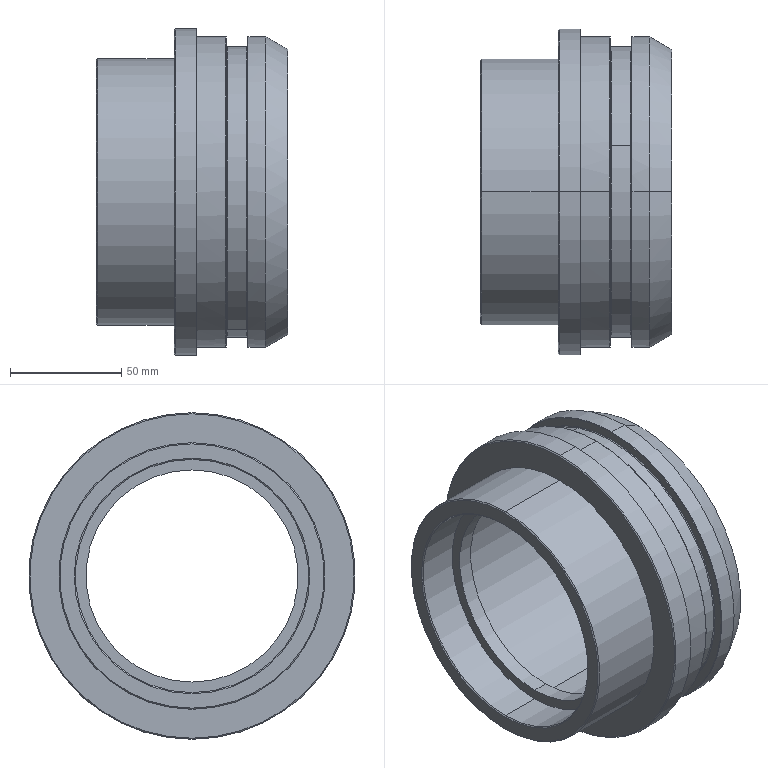Part | SolidWorks | features ICE 5, Chamfer 3, Cavity 1, Extrusion 1 | 1 solid | 42 faces | box 86 x 147 x 147 mm | volume 431094 mm3 | cylinder 16 | cone 10 | torus 8 | plane 8 | commonest cylinder face diameters 105 x4 140 x4 95.5 x2 120 x2 131 x2 147 x2
STEP:
#1=CARTESIAN_POINT('',(0.,0.,59.5));
#2=VERTEX_POINT('',#1);
#3=CARTESIAN_POINT('',(0.,0.,-59.5));
#4=VERTEX_POINT('',#3);
#5=CARTESIAN_POINT('',(0.,0.,0.));
#6=DIRECTION('',(-1.,0.,0.));
#7=DIRECTION('',(0.,0.,-1.));
#8=AXIS2_PLACEMENT_3D('',#5,#6,#7);
#9=CIRCLE('',#8,59.5);
#10=EDGE_CURVE('',#2,#4,#9,.T.);
#11=ORIENTED_EDGE('',*,*,#10,.F.);
#12=CARTESIAN_POINT('',(0.5,0.,60.));
#13=VERTEX_POINT('',#12);
#14=CARTESIAN_POINT('',(0.,0.,59.5));
#15=DIRECTION('',(0.7071,0.,0.7071));
#16=VECTOR('',#15,1000.);
#17=LINE('',#14,#16);
#18=EDGE_CURVE('',#2,#13,#17,.T.);
#19=ORIENTED_EDGE('',*,*,#18,.T.);
#20=CARTESIAN_POINT('',(0.5,0.,-60.));
#21=VERTEX_POINT('',#20);
#22=CARTESIAN_POINT('',(0.5,0.,0.));
#23=DIRECTION('',(1.,0.,0.));
#24=DIRECTION('',(0.,0.,-1.));
#25=AXIS2_PLACEMENT_3D('',#22,#23,#24);
#26=CIRCLE('',#25,60.);
#27=EDGE_CURVE('',#21,#13,#26,.T.);
#28=ORIENTED_EDGE('',*,*,#27,.F.);
#29=CARTESIAN_POINT('',(0.,0.,-59.5));
#30=DIRECTION('',(0.7071,0.,-0.7071));
#31=VECTOR('',#30,1000.);
#32=LINE('',#29,#31);
#33=EDGE_CURVE('',#4,#21,#32,.T.);
#34=ORIENTED_EDGE('',*,*,#33,.F.);
#35=EDGE_LOOP('',(#11,#19,#28,#34));
#36=FACE_OUTER_BOUND('',#35,.T.);
#37=CARTESIAN_POINT('',(0.,0.,0.));
#38=DIRECTION('',(1.,0.,0.));
#39=DIRECTION('',(0.,0.,-1.));
#40=AXIS2_PLACEMENT_3D('',#37,#38,#39);
#41=CONICAL_SURFACE('',#40,59.5,0.7854);
#42=ADVANCED_FACE('',(#36),#41,.T.);
#43=CARTESIAN_POINT('',(35.,0.,73.));
#44=VERTEX_POINT('',#43);
#45=CARTESIAN_POINT('',(35.,0.,-73.));
#46=VERTEX_POINT('',#45);
#47=CARTESIAN_POINT('',(35.,0.,0.));
#48=DIRECTION('',(-1.,0.,0.));
#49=DIRECTION('',(0.,0.,1.));
#50=AXIS2_PLACEMENT_3D('',#47,#48,#49);
#51=CIRCLE('',#50,73.);
#52=EDGE_CURVE('',#44,#46,#51,.T.);
#53=ORIENTED_EDGE('',*,*,#52,.F.);
#54=CARTESIAN_POINT('',(35.5,0.,73.5));
#55=VERTEX_POINT('',#54);
#56=CARTESIAN_POINT('',(35.,0.,73.));
#57=DIRECTION('',(0.7071,0.,0.7071));
#58=VECTOR('',#57,1000.);
#59=LINE('',#56,#58);
#60=EDGE_CURVE('',#44,#55,#59,.T.);
#61=ORIENTED_EDGE('',*,*,#60,.T.);
#62=CARTESIAN_POINT('',(35.5,0.,-73.5));
#63=VERTEX_POINT('',#62);
#64=CARTESIAN_POINT('',(35.5,0.,0.));
#65=DIRECTION('',(1.,0.,0.));
#66=DIRECTION('',(0.,0.,1.));
#67=AXIS2_PLACEMENT_3D('',#64,#65,#66);
#68=CIRCLE('',#67,73.5);
#69=EDGE_CURVE('',#63,#55,#68,.T.);
#70=ORIENTED_EDGE('',*,*,#69,.F.);
#71=CARTESIAN_POINT('',(35.,0.,-73.));
#72=DIRECTION('',(0.7071,0.,-0.7071));
#73=VECTOR('',#72,1000.);
#74=LINE('',#71,#73);
#75=EDGE_CURVE('',#46,#63,#74,.T.);
#76=ORIENTED_EDGE('',*,*,#75,.F.);
#77=EDGE_LOOP('',(#53,#61,#70,#76));
#78=FACE_OUTER_BOUND('',#77,.T.);
#79=CARTESIAN_POINT('',(35.,0.,0.));
#80=DIRECTION('',(1.,0.,0.));
#81=DIRECTION('',(0.,0.,-1.));
#82=AXIS2_PLACEMENT_3D('',#79,#80,#81);
#83=CONICAL_SURFACE('',#82,73.,0.7854);
#84=ADVANCED_FACE('',(#78),#83,.T.);
#85=CARTESIAN_POINT('',(0.5,0.,-52.5));
#86=VERTEX_POINT('',#85);
#87=CARTESIAN_POINT('',(0.5,0.,52.5));
#88=VERTEX_POINT('',#87);
#89=CARTESIAN_POINT('',(0.5,0.,0.));
#90=DIRECTION('',(-1.,0.,0.));
#91=DIRECTION('',(0.,0.,-1.));
#92=AXIS2_PLACEMENT_3D('',#89,#90,#91);
#93=CIRCLE('',#92,52.5);
#94=EDGE_CURVE('',#86,#88,#93,.T.);
#95=ORIENTED_EDGE('',*,*,#94,.F.);
#96=CARTESIAN_POINT('',(0.,0.,-53.));
#97=VERTEX_POINT('',#96);
#98=CARTESIAN_POINT('',(0.5,0.,-52.5));
#99=DIRECTION('',(-0.7071,0.,-0.7071));
#100=VECTOR('',#99,1000.);
#101=LINE('',#98,#100);
#102=EDGE_CURVE('',#86,#97,#101,.T.);
#103=ORIENTED_EDGE('',*,*,#102,.T.);
#104=CARTESIAN_POINT('',(0.,0.,53.));
#105=VERTEX_POINT('',#104);
#106=CARTESIAN_POINT('',(0.,0.,0.));
#107=DIRECTION('',(1.,0.,0.));
#108=DIRECTION('',(0.,0.,-1.));
#109=AXIS2_PLACEMENT_3D('',#106,#107,#108);
#110=CIRCLE('',#109,53.);
#111=EDGE_CURVE('',#105,#97,#110,.T.);
#112=ORIENTED_EDGE('',*,*,#111,.F.);
#113=CARTESIAN_POINT('',(0.5,0.,52.5));
#114=DIRECTION('',(-0.7071,0.,0.7071));
#115=VECTOR('',#114,1000.);
#116=LINE('',#113,#115);
#117=EDGE_CURVE('',#88,#105,#116,.T.);
#118=ORIENTED_EDGE('',*,*,#117,.F.);
#119=EDGE_LOOP('',(#95,#103,#112,#118));
#120=FACE_OUTER_BOUND('',#119,.T.);
#121=CARTESIAN_POINT('',(0.5,0.,0.));
#122=DIRECTION('',(-1.,0.,0.));
#123=DIRECTION('',(0.,0.,1.));
#124=AXIS2_PLACEMENT_3D('',#121,#122,#123);
#125=CONICAL_SURFACE('',#124,52.5,0.7854);
#126=ADVANCED_FACE('',(#120),#125,.F.);
#127=CARTESIAN_POINT('',(35.,0.,60.));
#128=VERTEX_POINT('',#127);
#129=CARTESIAN_POINT('',(35.,0.,-60.));
#130=VERTEX_POINT('',#129);
#131=CARTESIAN_POINT('',(35.,0.,0.));
#132=DIRECTION('',(-1.,0.,0.));
#133=DIRECTION('',(0.,0.,1.));
#134=AXIS2_PLACEMENT_3D('',#131,#132,#133);
#135=CIRCLE('',#134,60.);
#136=EDGE_CURVE('',#128,#130,#135,.T.);
#137=ORIENTED_EDGE('',*,*,#136,.T.);
#138=CARTESIAN_POINT('',(35.,0.,-60.));
#139=DIRECTION('',(-1.,0.,0.));
#140=VECTOR('',#139,1000.);
#141=LINE('',#138,#140);
#142=EDGE_CURVE('',#130,#21,#141,.T.);
#143=ORIENTED_EDGE('',*,*,#142,.T.);
#144=ORIENTED_EDGE('',*,*,#27,.T.);
#145=CARTESIAN_POINT('',(35.,0.,60.));
#146=DIRECTION('',(-1.,0.,0.));
#147=VECTOR('',#146,1000.);
#148=LINE('',#145,#147);
#149=EDGE_CURVE('',#128,#13,#148,.T.);
#150=ORIENTED_EDGE('',*,*,#149,.F.);
#151=EDGE_LOOP('',(#137,#143,#144,#150));
#152=FACE_OUTER_BOUND('',#151,.T.);
#153=CARTESIAN_POINT('',(35.,0.,0.));
#154=DIRECTION('',(-1.,0.,0.));
#155=DIRECTION('',(0.,0.,1.));
#156=AXIS2_PLACEMENT_3D('',#153,#154,#155);
#157=CYLINDRICAL_SURFACE('',#156,60.);
#158=ADVANCED_FACE('',(#152),#157,.T.);
#159=CARTESIAN_POINT('',(58.4,-22.387,-66.113));
#160=VERTEX_POINT('',#159);
#161=CARTESIAN_POINT('',(58.4,22.387,66.113));
#162=VERTEX_POINT('',#161);
#163=CARTESIAN_POINT('',(58.4,0.,0.));
#164=DIRECTION('',(-1.,0.,0.));
#165=DIRECTION('',(0.,-0.3207,-0.9472));
#166=AXIS2_PLACEMENT_3D('',#163,#164,#165);
#167=CIRCLE('',#166,69.8);
#168=EDGE_CURVE('',#160,#162,#167,.T.);
#169=ORIENTED_EDGE('',*,*,#168,.T.);
#170=CARTESIAN_POINT('',(58.2,22.451,66.302));
#171=VERTEX_POINT('',#170);
#172=CARTESIAN_POINT('',(58.2,22.387,66.113));
#173=DIRECTION('',(0.,-0.9472,0.3207));
#174=DIRECTION('',(0.,-0.3207,-0.9472));
#175=AXIS2_PLACEMENT_3D('',#172,#173,#174);
#176=CIRCLE('',#175,0.2);
#177=EDGE_CURVE('',#162,#171,#176,.T.);
#178=ORIENTED_EDGE('',*,*,#177,.T.);
#179=CARTESIAN_POINT('',(58.2,0.,70.));
#180=VERTEX_POINT('',#179);
#181=CARTESIAN_POINT('',(58.2,0.,0.));
#182=DIRECTION('',(-1.,0.,0.));
#183=DIRECTION('',(0.,-0.3207,-0.9472));
#184=AXIS2_PLACEMENT_3D('',#181,#182,#183);
#185=CIRCLE('',#184,70.);
#186=EDGE_CURVE('',#180,#171,#185,.T.);
#187=ORIENTED_EDGE('',*,*,#186,.F.);
#188=CARTESIAN_POINT('',(58.2,-22.451,-66.302));
#189=VERTEX_POINT('',#188);
#190=CARTESIAN_POINT('',(58.2,0.,0.));
#191=DIRECTION('',(-1.,0.,0.));
#192=DIRECTION('',(0.,-0.3207,-0.9472));
#193=AXIS2_PLACEMENT_3D('',#190,#191,#192);
#194=CIRCLE('',#193,70.);
#195=EDGE_CURVE('',#189,#180,#194,.T.);
#196=ORIENTED_EDGE('',*,*,#195,.F.);
#197=CARTESIAN_POINT('',(58.2,-22.387,-66.113));
#198=DIRECTION('',(0.,0.9472,-0.3207));
#199=DIRECTION('',(0.,0.3207,0.9472));
#200=AXIS2_PLACEMENT_3D('',#197,#198,#199);
#201=CIRCLE('',#200,0.2);
#202=EDGE_CURVE('',#160,#189,#201,.T.);
#203=ORIENTED_EDGE('',*,*,#202,.F.);
#204=EDGE_LOOP('',(#169,#178,#187,#196,#203));
#205=FACE_OUTER_BOUND('',#204,.T.);
#206=CARTESIAN_POINT('',(58.2,0.,0.));
#207=DIRECTION('',(-1.,0.,0.));
#208=DIRECTION('',(0.,-0.3207,-0.9472));
#209=AXIS2_PLACEMENT_3D('',#206,#207,#208);
#210=TOROIDAL_SURFACE('',#209,69.8,0.2);
#211=ADVANCED_FACE('',(#205),#210,.T.);
#212=CARTESIAN_POINT('',(68.2,0.,70.));
#213=VERTEX_POINT('',#212);
#214=CARTESIAN_POINT('',(68.2,22.451,66.302));
#215=VERTEX_POINT('',#214);
#216=CARTESIAN_POINT('',(68.2,0.,0.));
#217=DIRECTION('',(-1.,0.,0.));
#218=DIRECTION('',(0.,-0.3207,-0.9472));
#219=AXIS2_PLACEMENT_3D('',#216,#217,#218);
#220=CIRCLE('',#219,70.);
#221=EDGE_CURVE('',#213,#215,#220,.T.);
#222=ORIENTED_EDGE('',*,*,#221,.T.);
#223=CARTESIAN_POINT('',(68.,22.387,66.113));
#224=VERTEX_POINT('',#223);
#225=CARTESIAN_POINT('',(68.2,22.387,66.113));
#226=DIRECTION('',(0.,-0.9472,0.3207));
#227=DIRECTION('',(0.,-0.3207,-0.9472));
#228=AXIS2_PLACEMENT_3D('',#225,#226,#227);
#229=CIRCLE('',#228,0.2);
#230=EDGE_CURVE('',#215,#224,#229,.T.);
#231=ORIENTED_EDGE('',*,*,#230,.T.);
#232=CARTESIAN_POINT('',(68.,-22.387,-66.113));
#233=VERTEX_POINT('',#232);
#234=CARTESIAN_POINT('',(68.,0.,0.));
#235=DIRECTION('',(-1.,0.,0.));
#236=DIRECTION('',(0.,-0.3207,-0.9472));
#237=AXIS2_PLACEMENT_3D('',#234,#235,#236);
#238=CIRCLE('',#237,69.8);
#239=EDGE_CURVE('',#233,#224,#238,.T.);
#240=ORIENTED_EDGE('',*,*,#239,.F.);
#241=CARTESIAN_POINT('',(68.2,-22.451,-66.302));
#242=VERTEX_POINT('',#241);
#243=CARTESIAN_POINT('',(68.2,-22.387,-66.113));
#244=DIRECTION('',(0.,0.9472,-0.3207));
#245=DIRECTION('',(0.,0.3207,0.9472));
#246=AXIS2_PLACEMENT_3D('',#243,#244,#245);
#247=CIRCLE('',#246,0.2);
#248=EDGE_CURVE('',#242,#233,#247,.T.);
#249=ORIENTED_EDGE('',*,*,#248,.F.);
#250=CARTESIAN_POINT('',(68.2,0.,0.));
#251=DIRECTION('',(-1.,0.,0.));
#252=DIRECTION('',(0.,-0.3207,-0.9472));
#253=AXIS2_PLACEMENT_3D('',#250,#251,#252);
#254=CIRCLE('',#253,70.);
#255=EDGE_CURVE('',#242,#213,#254,.T.);
#256=ORIENTED_EDGE('',*,*,#255,.T.);
#257=EDGE_LOOP('',(#222,#231,#240,#249,#256));
#258=FACE_OUTER_BOUND('',#257,.T.);
#259=CARTESIAN_POINT('',(68.2,0.,0.));
#260=DIRECTION('',(-1.,0.,0.));
#261=DIRECTION('',(0.,-0.3207,-0.9472));
#262=AXIS2_PLACEMENT_3D('',#259,#260,#261);
#263=TOROIDAL_SURFACE('',#262,69.8,0.2);
#264=ADVANCED_FACE('',(#258),#263,.T.);
#265=CARTESIAN_POINT('',(67.6,21.007,62.04));
#266=VERTEX_POINT('',#265);
#267=CARTESIAN_POINT('',(67.6,-21.007,-62.04));
#268=VERTEX_POINT('',#267);
#269=CARTESIAN_POINT('',(67.6,0.,0.));
#270=DIRECTION('',(-1.,0.,0.));
#271=DIRECTION('',(0.,-0.3207,-0.9472));
#272=AXIS2_PLACEMENT_3D('',#269,#270,#271);
#273=CIRCLE('',#272,65.5);
#274=EDGE_CURVE('',#266,#268,#273,.T.);
#275=ORIENTED_EDGE('',*,*,#274,.F.);
#276=CARTESIAN_POINT('',(68.,21.136,62.419));
#277=VERTEX_POINT('',#276);
#278=CARTESIAN_POINT('',(67.6,21.136,62.419));
#279=DIRECTION('',(0.,-0.9472,0.3207));
#280=DIRECTION('',(0.,-0.3207,-0.9472));
#281=AXIS2_PLACEMENT_3D('',#278,#279,#280);
#282=CIRCLE('',#281,0.4);
#283=EDGE_CURVE('',#266,#277,#282,.T.);
#284=ORIENTED_EDGE('',*,*,#283,.T.);
#285=CARTESIAN_POINT('',(68.,-21.136,-62.419));
#286=VERTEX_POINT('',#285);
#287=CARTESIAN_POINT('',(68.,0.,0.));
#288=DIRECTION('',(-1.,0.,0.));
#289=DIRECTION('',(0.,-0.3207,-0.9472));
#290=AXIS2_PLACEMENT_3D('',#287,#288,#289);
#291=CIRCLE('',#290,65.9);
#292=EDGE_CURVE('',#277,#286,#291,.T.);
#293=ORIENTED_EDGE('',*,*,#292,.T.);
#294=CARTESIAN_POINT('',(67.6,-21.136,-62.419));
#295=DIRECTION('',(0.,0.9472,-0.3207));
#296=DIRECTION('',(0.,0.3207,0.9472));
#297=AXIS2_PLACEMENT_3D('',#294,#295,#296);
#298=CIRCLE('',#297,0.4);
#299=EDGE_CURVE('',#268,#286,#298,.T.);
#300=ORIENTED_EDGE('',*,*,#299,.F.);
#301=EDGE_LOOP('',(#275,#284,#293,#300));
#302=FACE_OUTER_BOUND('',#301,.T.);
#303=CARTESIAN_POINT('',(67.6,0.,0.));
#304=DIRECTION('',(-1.,0.,0.));
#305=DIRECTION('',(0.,-0.3207,-0.9472));
#306=AXIS2_PLACEMENT_3D('',#303,#304,#305);
#307=TOROIDAL_SURFACE('',#306,65.9,0.4);
#308=ADVANCED_FACE('',(#302),#307,.F.);
#309=CARTESIAN_POINT('',(58.4,21.136,62.419));
#310=VERTEX_POINT('',#309);
#311=CARTESIAN_POINT('',(58.4,-21.136,-62.419));
#312=VERTEX_POINT('',#311);
#313=CARTESIAN_POINT('',(58.4,0.,0.));
#314=DIRECTION('',(-1.,0.,0.));
#315=DIRECTION('',(0.,-0.3207,-0.9472));
#316=AXIS2_PLACEMENT_3D('',#313,#314,#315);
#317=CIRCLE('',#316,65.9);
#318=EDGE_CURVE('',#310,#312,#317,.T.);
#319=ORIENTED_EDGE('',*,*,#318,.F.);
#320=CARTESIAN_POINT('',(58.8,21.007,62.04));
#321=VERTEX_POINT('',#320);
#322=CARTESIAN_POINT('',(58.8,21.136,62.419));
#323=DIRECTION('',(0.,-0.9472,0.3207));
#324=DIRECTION('',(0.,-0.3207,-0.9472));
#325=AXIS2_PLACEMENT_3D('',#322,#323,#324);
#326=CIRCLE('',#325,0.4);
#327=EDGE_CURVE('',#310,#321,#326,.T.);
#328=ORIENTED_EDGE('',*,*,#327,.T.);
#329=CARTESIAN_POINT('',(58.8,-21.007,-62.04));
#330=VERTEX_POINT('',#329);
#331=CARTESIAN_POINT('',(58.8,0.,0.));
#332=DIRECTION('',(-1.,0.,0.));
#333=DIRECTION('',(0.,-0.3207,-0.9472));
#334=AXIS2_PLACEMENT_3D('',#331,#332,#333);
#335=CIRCLE('',#334,65.5);
#336=EDGE_CURVE('',#321,#330,#335,.T.);
#337=ORIENTED_EDGE('',*,*,#336,.T.);
#338=CARTESIAN_POINT('',(58.8,-21.136,-62.419));
#339=DIRECTION('',(0.,0.9472,-0.3207));
#340=DIRECTION('',(0.,0.3207,0.9472));
#341=AXIS2_PLACEMENT_3D('',#338,#339,#340);
#342=CIRCLE('',#341,0.4);
#343=EDGE_CURVE('',#312,#330,#342,.T.);
#344=ORIENTED_EDGE('',*,*,#343,.F.);
#345=EDGE_LOOP('',(#319,#328,#337,#344));
#346=FACE_OUTER_BOUND('',#345,.T.);
#347=CARTESIAN_POINT('',(58.8,0.,0.));
#348=DIRECTION('',(-1.,0.,0.));
#349=DIRECTION('',(0.,-0.3207,-0.9472));
#350=AXIS2_PLACEMENT_3D('',#347,#348,#349);
#351=TOROIDAL_SURFACE('',#350,65.9,0.4);
#352=ADVANCED_FACE('',(#346),#351,.F.);
#353=CARTESIAN_POINT('',(67.6,0.,0.));
#354=DIRECTION('',(-1.,0.,0.));
#355=DIRECTION('',(0.,-0.3207,-0.9472));
#356=AXIS2_PLACEMENT_3D('',#353,#354,#355);
#357=CIRCLE('',#356,65.5);
#358=EDGE_CURVE('',#268,#266,#357,.T.);
#359=ORIENTED_EDGE('',*,*,#358,.T.);
#360=CARTESIAN_POINT('',(-106.64,21.007,62.04));
#361=DIRECTION('',(-1.,0.,0.));
#362=VECTOR('',#361,1000.);
#363=LINE('',#360,#362);
#364=EDGE_CURVE('',#266,#321,#363,.T.);
#365=ORIENTED_EDGE('',*,*,#364,.T.);
#366=CARTESIAN_POINT('',(58.8,0.,0.));
#367=DIRECTION('',(-1.,0.,0.));
#368=DIRECTION('',(0.,-0.3207,-0.9472));
#369=AXIS2_PLACEMENT_3D('',#366,#367,#368);
#370=CIRCLE('',#369,65.5);
#371=EDGE_CURVE('',#330,#321,#370,.T.);
#372=ORIENTED_EDGE('',*,*,#371,.F.);
#373=CARTESIAN_POINT('',(-106.64,-21.007,-62.04));
#374=DIRECTION('',(-1.,0.,0.));
#375=VECTOR('',#374,1000.);
#376=LINE('',#373,#375);
#377=EDGE_CURVE('',#268,#330,#376,.T.);
#378=ORIENTED_EDGE('',*,*,#377,.F.);
#379=EDGE_LOOP('',(#359,#365,#372,#378));
#380=FACE_OUTER_BOUND('',#379,.T.);
#381=CARTESIAN_POINT('',(-106.64,0.,0.));
#382=DIRECTION('',(-1.,0.,0.));
#383=DIRECTION('',(0.,-0.3207,-0.9472));
#384=AXIS2_PLACEMENT_3D('',#381,#382,#383);
#385=CYLINDRICAL_SURFACE('',#384,65.5);
#386=ADVANCED_FACE('',(#380),#385,.T.);
#387=CARTESIAN_POINT('',(83.,0.,52.5));
#388=VERTEX_POINT('',#387);
#389=CARTESIAN_POINT('',(83.,0.,-52.5));
#390=VERTEX_POINT('',#389);
#391=CARTESIAN_POINT('',(83.,0.,0.));
#392=DIRECTION('',(1.,0.,0.));
#393=DIRECTION('',(0.,0.,-1.));
#394=AXIS2_PLACEMENT_3D('',#391,#392,#393);
#395=CIRCLE('',#394,52.5);
#396=EDGE_CURVE('',#388,#390,#395,.T.);
#397=ORIENTED_EDGE('',*,*,#396,.F.);
#398=CARTESIAN_POINT('',(86.,0.,53.592));
#399=VERTEX_POINT('',#398);
#400=CARTESIAN_POINT('',(83.,0.,52.5));
#401=DIRECTION('',(0.9397,0.,0.342));
#402=VECTOR('',#401,1000.);
#403=LINE('',#400,#402);
#404=EDGE_CURVE('',#388,#399,#403,.T.);
#405=ORIENTED_EDGE('',*,*,#404,.T.);
#406=CARTESIAN_POINT('',(86.,0.,-53.592));
#407=VERTEX_POINT('',#406);
#408=CARTESIAN_POINT('',(86.,0.,0.));
#409=DIRECTION('',(-1.,0.,0.));
#410=DIRECTION('',(0.,0.,-1.));
#411=AXIS2_PLACEMENT_3D('',#408,#409,#410);
#412=CIRCLE('',#411,53.592);
#413=EDGE_CURVE('',#407,#399,#412,.T.);
#414=ORIENTED_EDGE('',*,*,#413,.F.);
#415=CARTESIAN_POINT('',(83.,0.,-52.5));
#416=DIRECTION('',(0.9397,0.,-0.342));
#417=VECTOR('',#416,1000.);
#418=LINE('',#415,#417);
#419=EDGE_CURVE('',#390,#407,#418,.T.);
#420=ORIENTED_EDGE('',*,*,#419,.F.);
#421=EDGE_LOOP('',(#397,#405,#414,#420));
#422=FACE_OUTER_BOUND('',#421,.T.);
#423=CARTESIAN_POINT('',(83.,0.,0.));
#424=DIRECTION('',(1.,0.,0.));
#425=DIRECTION('',(0.,0.,-1.));
#426=AXIS2_PLACEMENT_3D('',#423,#424,#425);
#427=CONICAL_SURFACE('',#426,52.5,0.3491);
#428=ADVANCED_FACE('',(#422),#427,.F.);
#429=CARTESIAN_POINT('',(86.,0.,-64.226));
#430=VERTEX_POINT('',#429);
#431=CARTESIAN_POINT('',(86.,0.,64.226));
#432=VERTEX_POINT('',#431);
#433=CARTESIAN_POINT('',(86.,0.,0.));
#434=DIRECTION('',(1.,0.,0.));
#435=DIRECTION('',(0.,0.,-1.));
#436=AXIS2_PLACEMENT_3D('',#433,#434,#435);
#437=CIRCLE('',#436,64.226);
#438=EDGE_CURVE('',#430,#432,#437,.T.);
#439=ORIENTED_EDGE('',*,*,#438,.F.);
#440=CARTESIAN_POINT('',(76.,0.,-70.));
#441=VERTEX_POINT('',#440);
#442=CARTESIAN_POINT('',(86.,0.,-64.226));
#443=DIRECTION('',(-0.866,0.,-0.5));
#444=VECTOR('',#443,1000.);
#445=LINE('',#442,#444);
#446=EDGE_CURVE('',#430,#441,#445,.T.);
#447=ORIENTED_EDGE('',*,*,#446,.T.);
#448=CARTESIAN_POINT('',(76.,0.,70.));
#449=VERTEX_POINT('',#448);
#450=CARTESIAN_POINT('',(76.,0.,0.));
#451=DIRECTION('',(-1.,0.,0.));
#452=DIRECTION('',(0.,0.,-1.));
#453=AXIS2_PLACEMENT_3D('',#450,#451,#452);
#454=CIRCLE('',#453,70.);
#455=EDGE_CURVE('',#449,#441,#454,.T.);
#456=ORIENTED_EDGE('',*,*,#455,.F.);
#457=CARTESIAN_POINT('',(86.,0.,64.226));
#458=DIRECTION('',(-0.866,0.,0.5));
#459=VECTOR('',#458,1000.);
#460=LINE('',#457,#459);
#461=EDGE_CURVE('',#432,#449,#460,.T.);
#462=ORIENTED_EDGE('',*,*,#461,.F.);
#463=EDGE_LOOP('',(#439,#447,#456,#462));
#464=FACE_OUTER_BOUND('',#463,.T.);
#465=CARTESIAN_POINT('',(86.,0.,0.));
#466=DIRECTION('',(-1.,0.,0.));
#467=DIRECTION('',(0.,0.,1.));
#468=AXIS2_PLACEMENT_3D('',#465,#466,#467);
#469=CONICAL_SURFACE('',#468,64.226,0.5236);
#470=ADVANCED_FACE('',(#464),#469,.T.);
#471=CARTESIAN_POINT('',(26.,0.,47.75));
#472=VERTEX_POINT('',#471);
#473=CARTESIAN_POINT('',(26.,0.,-47.75));
#474=VERTEX_POINT('',#473);
#475=CARTESIAN_POINT('',(26.,0.,0.));
#476=DIRECTION('',(1.,0.,0.));
#477=DIRECTION('',(0.,0.,-1.));
#478=AXIS2_PLACEMENT_3D('',#475,#476,#477);
#479=CIRCLE('',#478,47.75);
#480=EDGE_CURVE('',#472,#474,#479,.T.);
#481=ORIENTED_EDGE('',*,*,#480,.T.);
#482=CARTESIAN_POINT('',(19.,0.,-47.75));
#483=VERTEX_POINT('',#482);
#484=CARTESIAN_POINT('',(38.,0.,-47.75));
#485=DIRECTION('',(-1.,0.,0.));
#486=VECTOR('',#485,1000.);
#487=LINE('',#484,#486);
#488=EDGE_CURVE('',#474,#483,#487,.T.);
#489=ORIENTED_EDGE('',*,*,#488,.T.);
#490=CARTESIAN_POINT('',(19.,0.,47.75));
#491=VERTEX_POINT('',#490);
#492=CARTESIAN_POINT('',(19.,0.,0.));
#493=DIRECTION('',(-1.,0.,0.));
#494=DIRECTION('',(0.,0.,1.));
#495=AXIS2_PLACEMENT_3D('',#492,#493,#494);
#496=CIRCLE('',#495,47.75);
#497=EDGE_CURVE('',#483,#491,#496,.T.);
#498=ORIENTED_EDGE('',*,*,#497,.T.);
#499=CARTESIAN_POINT('',(38.,0.,47.75));
#500=DIRECTION('',(-1.,0.,0.));
#501=VECTOR('',#500,1000.);
#502=LINE('',#499,#501);
#503=EDGE_CURVE('',#472,#491,#502,.T.);
#504=ORIENTED_EDGE('',*,*,#503,.F.);
#505=EDGE_LOOP('',(#481,#489,#498,#504));
#506=FACE_OUTER_BOUND('',#505,.T.);
#507=CARTESIAN_POINT('',(38.,0.,0.));
#508=DIRECTION('',(-1.,0.,0.));
#509=DIRECTION('',(0.,0.,1.));
#510=AXIS2_PLACEMENT_3D('',#507,#508,#509);
#511=CYLINDRICAL_SURFACE('',#510,47.75);
#512=ADVANCED_FACE('',(#506),#511,.F.);
#513=CARTESIAN_POINT('',(19.,0.,-52.5));
#514=VERTEX_POINT('',#513);
#515=CARTESIAN_POINT('',(19.,0.,52.5));
#516=VERTEX_POINT('',#515);
#517=CARTESIAN_POINT('',(19.,0.,0.));
#518=DIRECTION('',(-1.,0.,0.));
#519=DIRECTION('',(0.,0.,1.));
#520=AXIS2_PLACEMENT_3D('',#517,#518,#519);
#521=CIRCLE('',#520,52.5);
#522=EDGE_CURVE('',#514,#516,#521,.T.);
#523=ORIENTED_EDGE('',*,*,#522,.F.);
#524=CARTESIAN_POINT('',(19.,0.,-52.5));
#525=DIRECTION('',(-1.,0.,0.));
#526=VECTOR('',#525,1000.);
#527=LINE('',#524,#526);
#528=EDGE_CURVE('',#514,#86,#527,.T.);
#529=ORIENTED_EDGE('',*,*,#528,.T.);
#530=ORIENTED_EDGE('',*,*,#94,.T.);
#531=CARTESIAN_POINT('',(19.,0.,52.5));
#532=DIRECTION('',(-1.,0.,0.));
#533=VECTOR('',#532,1000.);
#534=LINE('',#531,#533);
#535=EDGE_CURVE('',#516,#88,#534,.T.);
#536=ORIENTED_EDGE('',*,*,#535,.F.);
#537=EDGE_LOOP('',(#523,#529,#530,#536));
#538=FACE_OUTER_BOUND('',#537,.T.);
#539=CARTESIAN_POINT('',(19.,0.,0.));
#540=DIRECTION('',(-1.,0.,0.));
#541=DIRECTION('',(0.,0.,1.));
#542=AXIS2_PLACEMENT_3D('',#539,#540,#541);
#543=CYLINDRICAL_SURFACE('',#542,52.5);
#544=ADVANCED_FACE('',(#538),#543,.F.);
#545=CARTESIAN_POINT('',(26.,0.,52.5));
#546=VERTEX_POINT('',#545);
#547=CARTESIAN_POINT('',(26.,0.,-52.5));
#548=VERTEX_POINT('',#547);
#549=CARTESIAN_POINT('',(26.,0.,0.));
#550=DIRECTION('',(1.,0.,0.));
#551=DIRECTION('',(0.,0.,-1.));
#552=AXIS2_PLACEMENT_3D('',#549,#550,#551);
#553=CIRCLE('',#552,52.5);
#554=EDGE_CURVE('',#546,#548,#553,.T.);
#555=ORIENTED_EDGE('',*,*,#554,.F.);
#556=CARTESIAN_POINT('',(26.,0.,52.5));
#557=DIRECTION('',(1.,0.,0.));
#558=VECTOR('',#557,1000.);
#559=LINE('',#556,#558);
#560=EDGE_CURVE('',#546,#388,#559,.T.);
#561=ORIENTED_EDGE('',*,*,#560,.T.);
#562=ORIENTED_EDGE('',*,*,#396,.T.);
#563=CARTESIAN_POINT('',(26.,0.,-52.5));
#564=DIRECTION('',(1.,0.,0.));
#565=VECTOR('',#564,1000.);
#566=LINE('',#563,#565);
#567=EDGE_CURVE('',#548,#390,#566,.T.);
#568=ORIENTED_EDGE('',*,*,#567,.F.);
#569=EDGE_LOOP('',(#555,#561,#562,#568));
#570=FACE_OUTER_BOUND('',#569,.T.);
#571=CARTESIAN_POINT('',(26.,0.,0.));
#572=DIRECTION('',(1.,0.,0.));
#573=DIRECTION('',(0.,0.,-1.));
#574=AXIS2_PLACEMENT_3D('',#571,#572,#573);
#575=CYLINDRICAL_SURFACE('',#574,52.5);
#576=ADVANCED_FACE('',(#570),#575,.F.);
#577=CARTESIAN_POINT('',(45.,0.,70.));
#578=VERTEX_POINT('',#577);
#579=CARTESIAN_POINT('',(45.,0.,-70.));
#580=VERTEX_POINT('',#579);
#581=CARTESIAN_POINT('',(45.,0.,0.));
#582=DIRECTION('',(-1.,0.,0.));
#583=DIRECTION('',(0.,0.,-1.));
#584=AXIS2_PLACEMENT_3D('',#581,#582,#583);
#585=CIRCLE('',#584,70.);
#586=EDGE_CURVE('',#578,#580,#585,.T.);
#587=ORIENTED_EDGE('',*,*,#586,.F.);
#588=CARTESIAN_POINT('',(-209.968,0.,70.));
#589=DIRECTION('',(1.,0.,0.));
#590=VECTOR('',#589,1000.);
#591=LINE('',#588,#590);
#592=EDGE_CURVE('',#578,#180,#591,.T.);
#593=ORIENTED_EDGE('',*,*,#592,.T.);
#594=ORIENTED_EDGE('',*,*,#186,.T.);
#595=CARTESIAN_POINT('',(58.2,0.,-70.));
#596=VERTEX_POINT('',#595);
#597=CARTESIAN_POINT('',(58.2,0.,0.));
#598=DIRECTION('',(-1.,0.,0.));
#599=DIRECTION('',(0.,-0.3207,-0.9472));
#600=AXIS2_PLACEMENT_3D('',#597,#598,#599);
#601=CIRCLE('',#600,70.);
#602=EDGE_CURVE('',#171,#596,#601,.T.);
#603=ORIENTED_EDGE('',*,*,#602,.T.);
#604=CARTESIAN_POINT('',(-209.968,0.,-70.));
#605=DIRECTION('',(1.,0.,0.));
#606=VECTOR('',#605,1000.);
#607=LINE('',#604,#606);
#608=EDGE_CURVE('',#580,#596,#607,.T.);
#609=ORIENTED_EDGE('',*,*,#608,.F.);
#610=EDGE_LOOP('',(#587,#593,#594,#603,#609));
#611=FACE_OUTER_BOUND('',#610,.T.);
#612=CARTESIAN_POINT('',(-209.968,0.,0.));
#613=DIRECTION('',(1.,0.,0.));
#614=DIRECTION('',(0.,0.,-1.));
#615=AXIS2_PLACEMENT_3D('',#612,#613,#614);
#616=CYLINDRICAL_SURFACE('',#615,70.);
#617=ADVANCED_FACE('',(#611),#616,.T.);
#618=ORIENTED_EDGE('',*,*,#221,.F.);
#619=CARTESIAN_POINT('',(-209.968,0.,70.));
#620=DIRECTION('',(1.,0.,0.));
#621=VECTOR('',#620,1000.);
#622=LINE('',#619,#621);
#623=EDGE_CURVE('',#213,#449,#622,.T.);
#624=ORIENTED_EDGE('',*,*,#623,.T.);
#625=ORIENTED_EDGE('',*,*,#455,.T.);
#626=CARTESIAN_POINT('',(68.2,0.,-70.));
#627=VERTEX_POINT('',#626);
#628=CARTESIAN_POINT('',(-209.968,0.,-70.));
#629=DIRECTION('',(1.,0.,0.));
#630=VECTOR('',#629,1000.);
#631=LINE('',#628,#630);
#632=EDGE_CURVE('',#627,#441,#631,.T.);
#633=ORIENTED_EDGE('',*,*,#632,.F.);
#634=CARTESIAN_POINT('',(68.2,0.,0.));
#635=DIRECTION('',(-1.,0.,0.));
#636=DIRECTION('',(0.,-0.3207,-0.9472));
#637=AXIS2_PLACEMENT_3D('',#634,#635,#636);
#638=CIRCLE('',#637,70.);
#639=EDGE_CURVE('',#215,#627,#638,.T.);
#640=ORIENTED_EDGE('',*,*,#639,.F.);
#641=EDGE_LOOP('',(#618,#624,#625,#633,#640));
#642=FACE_OUTER_BOUND('',#641,.T.);
#643=CARTESIAN_POINT('',(-209.968,0.,0.));
#644=DIRECTION('',(1.,0.,0.));
#645=DIRECTION('',(0.,0.,-1.));
#646=AXIS2_PLACEMENT_3D('',#643,#644,#645);
#647=CYLINDRICAL_SURFACE('',#646,70.);
#648=ADVANCED_FACE('',(#642),#647,.T.);
#649=CARTESIAN_POINT('',(45.,0.,-73.5));
#650=VERTEX_POINT('',#649);
#651=CARTESIAN_POINT('',(45.,0.,73.5));
#652=VERTEX_POINT('',#651);
#653=CARTESIAN_POINT('',(45.,0.,0.));
#654=DIRECTION('',(1.,0.,0.));
#655=DIRECTION('',(0.,0.,-1.));
#656=AXIS2_PLACEMENT_3D('',#653,#654,#655);
#657=CIRCLE('',#656,73.5);
#658=EDGE_CURVE('',#650,#652,#657,.T.);
#659=ORIENTED_EDGE('',*,*,#658,.F.);
#660=CARTESIAN_POINT('',(86.,0.,-73.5));
#661=DIRECTION('',(-1.,0.,0.));
#662=VECTOR('',#661,1000.);
#663=LINE('',#660,#662);
#664=EDGE_CURVE('',#650,#63,#663,.T.);
#665=ORIENTED_EDGE('',*,*,#664,.T.);
#666=ORIENTED_EDGE('',*,*,#69,.T.);
#667=CARTESIAN_POINT('',(86.,0.,73.5));
#668=DIRECTION('',(-1.,0.,0.));
#669=VECTOR('',#668,1000.);
#670=LINE('',#667,#669);
#671=EDGE_CURVE('',#652,#55,#670,.T.);
#672=ORIENTED_EDGE('',*,*,#671,.F.);
#673=EDGE_LOOP('',(#659,#665,#666,#672));
#674=FACE_OUTER_BOUND('',#673,.T.);
#675=CARTESIAN_POINT('',(86.,0.,0.));
#676=DIRECTION('',(-1.,0.,0.));
#677=DIRECTION('',(0.,0.,1.));
#678=AXIS2_PLACEMENT_3D('',#675,#676,#677);
#679=CYLINDRICAL_SURFACE('',#678,73.5);
#680=ADVANCED_FACE('',(#674),#679,.T.);
#681=ORIENTED_EDGE('',*,*,#664,.F.);
#682=CARTESIAN_POINT('',(45.,0.,0.));
#683=DIRECTION('',(1.,0.,0.));
#684=DIRECTION('',(0.,0.,-1.));
#685=AXIS2_PLACEMENT_3D('',#682,#683,#684);
#686=CIRCLE('',#685,73.5);
#687=EDGE_CURVE('',#652,#650,#686,.T.);
#688=ORIENTED_EDGE('',*,*,#687,.F.);
#689=ORIENTED_EDGE('',*,*,#671,.T.);
#690=CARTESIAN_POINT('',(35.5,0.,0.));
#691=DIRECTION('',(1.,0.,0.));
#692=DIRECTION('',(0.,0.,1.));
#693=AXIS2_PLACEMENT_3D('',#690,#691,#692);
#694=CIRCLE('',#693,73.5);
#695=EDGE_CURVE('',#55,#63,#694,.T.);
#696=ORIENTED_EDGE('',*,*,#695,.T.);
#697=EDGE_LOOP('',(#681,#688,#689,#696));
#698=FACE_OUTER_BOUND('',#697,.T.);
#699=CARTESIAN_POINT('',(86.,0.,0.));
#700=DIRECTION('',(-1.,0.,0.));
#701=DIRECTION('',(0.,0.,1.));
#702=AXIS2_PLACEMENT_3D('',#699,#700,#701);
#703=CYLINDRICAL_SURFACE('',#702,73.5);
#704=ADVANCED_FACE('',(#698),#703,.T.);
#705=ORIENTED_EDGE('',*,*,#111,.T.);
#706=CARTESIAN_POINT('',(0.,0.,0.));
#707=DIRECTION('',(1.,0.,0.));
#708=DIRECTION('',(0.,0.,-1.));
#709=AXIS2_PLACEMENT_3D('',#706,#707,#708);
#710=CIRCLE('',#709,53.);
#711=EDGE_CURVE('',#97,#105,#710,.T.);
#712=ORIENTED_EDGE('',*,*,#711,.T.);
#713=EDGE_LOOP('',(#705,#712));
#714=FACE_BOUND('',#713,.T.);
#715=CARTESIAN_POINT('',(0.,0.,0.));
#716=DIRECTION('',(-1.,0.,0.));
#717=DIRECTION('',(0.,0.,-1.));
#718=AXIS2_PLACEMENT_3D('',#715,#716,#717);
#719=CIRCLE('',#718,59.5);
#720=EDGE_CURVE('',#4,#2,#719,.T.);
#721=ORIENTED_EDGE('',*,*,#720,.T.);
#722=ORIENTED_EDGE('',*,*,#10,.T.);
#723=EDGE_LOOP('',(#721,#722));
#724=FACE_OUTER_BOUND('',#723,.T.);
#725=CARTESIAN_POINT('',(0.,0.,0.));
#726=DIRECTION('',(1.,0.,0.));
#727=DIRECTION('',(0.,0.,-1.));
#728=AXIS2_PLACEMENT_3D('',#725,#726,#727);
#729=PLANE('',#728);
#730=ADVANCED_FACE('',(#714,#724),#729,.F.);
#731=ORIENTED_EDGE('',*,*,#623,.F.);
#732=ORIENTED_EDGE('',*,*,#255,.F.);
#733=CARTESIAN_POINT('',(68.2,0.,0.));
#734=DIRECTION('',(-1.,0.,0.));
#735=DIRECTION('',(0.,-0.3207,-0.9472));
#736=AXIS2_PLACEMENT_3D('',#733,#734,#735);
#737=CIRCLE('',#736,70.);
#738=EDGE_CURVE('',#627,#242,#737,.T.);
#739=ORIENTED_EDGE('',*,*,#738,.F.);
#740=ORIENTED_EDGE('',*,*,#632,.T.);
#741=CARTESIAN_POINT('',(76.,0.,0.));
#742=DIRECTION('',(-1.,0.,0.));
#743=DIRECTION('',(0.,0.,-1.));
#744=AXIS2_PLACEMENT_3D('',#741,#742,#743);
#745=CIRCLE('',#744,70.);
#746=EDGE_CURVE('',#441,#449,#745,.T.);
#747=ORIENTED_EDGE('',*,*,#746,.T.);
#748=EDGE_LOOP('',(#731,#732,#739,#740,#747));
#749=FACE_OUTER_BOUND('',#748,.T.);
#750=CARTESIAN_POINT('',(-209.968,0.,0.));
#751=DIRECTION('',(1.,0.,0.));
#752=DIRECTION('',(0.,0.,-1.));
#753=AXIS2_PLACEMENT_3D('',#750,#751,#752);
#754=CYLINDRICAL_SURFACE('',#753,70.);
#755=ADVANCED_FACE('',(#749),#754,.T.);
#756=ORIENTED_EDGE('',*,*,#413,.T.);
#757=CARTESIAN_POINT('',(86.,0.,0.));
#758=DIRECTION('',(-1.,0.,0.));
#759=DIRECTION('',(0.,0.,-1.));
#760=AXIS2_PLACEMENT_3D('',#757,#758,#759);
#761=CIRCLE('',#760,53.592);
#762=EDGE_CURVE('',#399,#407,#761,.T.);
#763=ORIENTED_EDGE('',*,*,#762,.T.);
#764=EDGE_LOOP('',(#756,#763));
#765=FACE_BOUND('',#764,.T.);
#766=CARTESIAN_POINT('',(86.,0.,0.));
#767=DIRECTION('',(1.,0.,0.));
#768=DIRECTION('',(0.,0.,-1.));
#769=AXIS2_PLACEMENT_3D('',#766,#767,#768);
#770=CIRCLE('',#769,64.226);
#771=EDGE_CURVE('',#432,#430,#770,.T.);
#772=ORIENTED_EDGE('',*,*,#771,.T.);
#773=ORIENTED_EDGE('',*,*,#438,.T.);
#774=EDGE_LOOP('',(#772,#773));
#775=FACE_OUTER_BOUND('',#774,.T.);
#776=CARTESIAN_POINT('',(86.,0.,0.));
#777=DIRECTION('',(1.,0.,0.));
#778=DIRECTION('',(0.,0.,-1.));
#779=AXIS2_PLACEMENT_3D('',#776,#777,#778);
#780=PLANE('',#779);
#781=ADVANCED_FACE('',(#765,#775),#780,.T.);
#782=CARTESIAN_POINT('',(45.,0.,0.));
#783=DIRECTION('',(-1.,0.,0.));
#784=DIRECTION('',(0.,0.,-1.));
#785=AXIS2_PLACEMENT_3D('',#782,#783,#784);
#786=CIRCLE('',#785,70.);
#787=EDGE_CURVE('',#580,#578,#786,.T.);
#788=ORIENTED_EDGE('',*,*,#787,.T.);
#789=ORIENTED_EDGE('',*,*,#586,.T.);
#790=EDGE_LOOP('',(#788,#789));
#791=FACE_BOUND('',#790,.T.);
#792=ORIENTED_EDGE('',*,*,#687,.T.);
#793=ORIENTED_EDGE('',*,*,#658,.T.);
#794=EDGE_LOOP('',(#792,#793));
#795=FACE_OUTER_BOUND('',#794,.T.);
#796=CARTESIAN_POINT('',(45.,0.,0.));
#797=DIRECTION('',(1.,0.,0.));
#798=DIRECTION('',(0.,0.,-1.));
#799=AXIS2_PLACEMENT_3D('',#796,#797,#798);
#800=PLANE('',#799);
#801=ADVANCED_FACE('',(#791,#795),#800,.T.);
#802=ORIENTED_EDGE('',*,*,#592,.F.);
#803=ORIENTED_EDGE('',*,*,#787,.F.);
#804=ORIENTED_EDGE('',*,*,#608,.T.);
#805=CARTESIAN_POINT('',(58.2,0.,0.));
#806=DIRECTION('',(-1.,0.,0.));
#807=DIRECTION('',(0.,-0.3207,-0.9472));
#808=AXIS2_PLACEMENT_3D('',#805,#806,#807);
#809=CIRCLE('',#808,70.);
#810=EDGE_CURVE('',#596,#189,#809,.T.);
#811=ORIENTED_EDGE('',*,*,#810,.T.);
#812=ORIENTED_EDGE('',*,*,#195,.T.);
#813=EDGE_LOOP('',(#802,#803,#804,#811,#812));
#814=FACE_OUTER_BOUND('',#813,.T.);
#815=CARTESIAN_POINT('',(-209.968,0.,0.));
#816=DIRECTION('',(1.,0.,0.));
#817=DIRECTION('',(0.,0.,-1.));
#818=AXIS2_PLACEMENT_3D('',#815,#816,#817);
#819=CYLINDRICAL_SURFACE('',#818,70.);
#820=ADVANCED_FACE('',(#814),#819,.T.);
#821=ORIENTED_EDGE('',*,*,#560,.F.);
#822=CARTESIAN_POINT('',(26.,0.,0.));
#823=DIRECTION('',(1.,0.,0.));
#824=DIRECTION('',(0.,0.,-1.));
#825=AXIS2_PLACEMENT_3D('',#822,#823,#824);
#826=CIRCLE('',#825,52.5);
#827=EDGE_CURVE('',#548,#546,#826,.T.);
#828=ORIENTED_EDGE('',*,*,#827,.F.);
#829=ORIENTED_EDGE('',*,*,#567,.T.);
#830=CARTESIAN_POINT('',(83.,0.,0.));
#831=DIRECTION('',(1.,0.,0.));
#832=DIRECTION('',(0.,0.,-1.));
#833=AXIS2_PLACEMENT_3D('',#830,#831,#832);
#834=CIRCLE('',#833,52.5);
#835=EDGE_CURVE('',#390,#388,#834,.T.);
#836=ORIENTED_EDGE('',*,*,#835,.T.);
#837=EDGE_LOOP('',(#821,#828,#829,#836));
#838=FACE_OUTER_BOUND('',#837,.T.);
#839=CARTESIAN_POINT('',(26.,0.,0.));
#840=DIRECTION('',(1.,0.,0.));
#841=DIRECTION('',(0.,0.,-1.));
#842=AXIS2_PLACEMENT_3D('',#839,#840,#841);
#843=CYLINDRICAL_SURFACE('',#842,52.5);
#844=ADVANCED_FACE('',(#838),#843,.F.);
#845=ORIENTED_EDGE('',*,*,#480,.F.);
#846=CARTESIAN_POINT('',(26.,0.,0.));
#847=DIRECTION('',(1.,0.,0.));
#848=DIRECTION('',(0.,0.,-1.));
#849=AXIS2_PLACEMENT_3D('',#846,#847,#848);
#850=CIRCLE('',#849,47.75);
#851=EDGE_CURVE('',#474,#472,#850,.T.);
#852=ORIENTED_EDGE('',*,*,#851,.F.);
#853=EDGE_LOOP('',(#845,#852));
#854=FACE_BOUND('',#853,.T.);
#855=ORIENTED_EDGE('',*,*,#827,.T.);
#856=ORIENTED_EDGE('',*,*,#554,.T.);
#857=EDGE_LOOP('',(#855,#856));
#858=FACE_OUTER_BOUND('',#857,.T.);
#859=CARTESIAN_POINT('',(26.,0.,0.));
#860=DIRECTION('',(1.,0.,0.));
#861=DIRECTION('',(0.,0.,-1.));
#862=AXIS2_PLACEMENT_3D('',#859,#860,#861);
#863=PLANE('',#862);
#864=ADVANCED_FACE('',(#854,#858),#863,.T.);
#865=ORIENTED_EDGE('',*,*,#528,.F.);
#866=CARTESIAN_POINT('',(19.,0.,0.));
#867=DIRECTION('',(-1.,0.,0.));
#868=DIRECTION('',(0.,0.,1.));
#869=AXIS2_PLACEMENT_3D('',#866,#867,#868);
#870=CIRCLE('',#869,52.5);
#871=EDGE_CURVE('',#516,#514,#870,.T.);
#872=ORIENTED_EDGE('',*,*,#871,.F.);
#873=ORIENTED_EDGE('',*,*,#535,.T.);
#874=CARTESIAN_POINT('',(0.5,0.,0.));
#875=DIRECTION('',(-1.,0.,0.));
#876=DIRECTION('',(0.,0.,-1.));
#877=AXIS2_PLACEMENT_3D('',#874,#875,#876);
#878=CIRCLE('',#877,52.5);
#879=EDGE_CURVE('',#88,#86,#878,.T.);
#880=ORIENTED_EDGE('',*,*,#879,.T.);
#881=EDGE_LOOP('',(#865,#872,#873,#880));
#882=FACE_OUTER_BOUND('',#881,.T.);
#883=CARTESIAN_POINT('',(19.,0.,0.));
#884=DIRECTION('',(-1.,0.,0.));
#885=DIRECTION('',(0.,0.,1.));
#886=AXIS2_PLACEMENT_3D('',#883,#884,#885);
#887=CYLINDRICAL_SURFACE('',#886,52.5);
#888=ADVANCED_FACE('',(#882),#887,.F.);
#889=CARTESIAN_POINT('',(19.,0.,0.));
#890=DIRECTION('',(-1.,0.,0.));
#891=DIRECTION('',(0.,0.,1.));
#892=AXIS2_PLACEMENT_3D('',#889,#890,#891);
#893=CIRCLE('',#892,47.75);
#894=EDGE_CURVE('',#491,#483,#893,.T.);
#895=ORIENTED_EDGE('',*,*,#894,.F.);
#896=ORIENTED_EDGE('',*,*,#497,.F.);
#897=EDGE_LOOP('',(#895,#896));
#898=FACE_BOUND('',#897,.T.);
#899=ORIENTED_EDGE('',*,*,#871,.T.);
#900=ORIENTED_EDGE('',*,*,#522,.T.);
#901=EDGE_LOOP('',(#899,#900));
#902=FACE_OUTER_BOUND('',#901,.T.);
#903=CARTESIAN_POINT('',(19.,0.,0.));
#904=DIRECTION('',(-1.,0.,0.));
#905=DIRECTION('',(0.,0.,1.));
#906=AXIS2_PLACEMENT_3D('',#903,#904,#905);
#907=PLANE('',#906);
#908=ADVANCED_FACE('',(#898,#902),#907,.T.);
#909=ORIENTED_EDGE('',*,*,#488,.F.);
#910=ORIENTED_EDGE('',*,*,#851,.T.);
#911=ORIENTED_EDGE('',*,*,#503,.T.);
#912=ORIENTED_EDGE('',*,*,#894,.T.);
#913=EDGE_LOOP('',(#909,#910,#911,#912));
#914=FACE_OUTER_BOUND('',#913,.T.);
#915=CARTESIAN_POINT('',(38.,0.,0.));
#916=DIRECTION('',(-1.,0.,0.));
#917=DIRECTION('',(0.,0.,1.));
#918=AXIS2_PLACEMENT_3D('',#915,#916,#917);
#919=CYLINDRICAL_SURFACE('',#918,47.75);
#920=ADVANCED_FACE('',(#914),#919,.F.);
#921=ORIENTED_EDGE('',*,*,#446,.F.);
#922=ORIENTED_EDGE('',*,*,#771,.F.);
#923=ORIENTED_EDGE('',*,*,#461,.T.);
#924=ORIENTED_EDGE('',*,*,#746,.F.);
#925=EDGE_LOOP('',(#921,#922,#923,#924));
#926=FACE_OUTER_BOUND('',#925,.T.);
#927=CARTESIAN_POINT('',(86.,0.,0.));
#928=DIRECTION('',(-1.,0.,0.));
#929=DIRECTION('',(0.,0.,1.));
#930=AXIS2_PLACEMENT_3D('',#927,#928,#929);
#931=CONICAL_SURFACE('',#930,64.226,0.5236);
#932=ADVANCED_FACE('',(#926),#931,.T.);
#933=ORIENTED_EDGE('',*,*,#404,.F.);
#934=ORIENTED_EDGE('',*,*,#835,.F.);
#935=ORIENTED_EDGE('',*,*,#419,.T.);
#936=ORIENTED_EDGE('',*,*,#762,.F.);
#937=EDGE_LOOP('',(#933,#934,#935,#936));
#938=FACE_OUTER_BOUND('',#937,.T.);
#939=CARTESIAN_POINT('',(83.,0.,0.));
#940=DIRECTION('',(1.,0.,0.));
#941=DIRECTION('',(0.,0.,-1.));
#942=AXIS2_PLACEMENT_3D('',#939,#940,#941);
#943=CONICAL_SURFACE('',#942,52.5,0.3491);
#944=ADVANCED_FACE('',(#938),#943,.F.);
#945=ORIENTED_EDGE('',*,*,#364,.F.);
#946=ORIENTED_EDGE('',*,*,#274,.T.);
#947=ORIENTED_EDGE('',*,*,#377,.T.);
#948=ORIENTED_EDGE('',*,*,#336,.F.);
#949=EDGE_LOOP('',(#945,#946,#947,#948));
#950=FACE_OUTER_BOUND('',#949,.T.);
#951=CARTESIAN_POINT('',(-106.64,0.,0.));
#952=DIRECTION('',(-1.,0.,0.));
#953=DIRECTION('',(0.,-0.3207,-0.9472));
#954=AXIS2_PLACEMENT_3D('',#951,#952,#953);
#955=CYLINDRICAL_SURFACE('',#954,65.5);
#956=ADVANCED_FACE('',(#950),#955,.T.);
#957=CARTESIAN_POINT('',(68.,0.,0.));
#958=DIRECTION('',(-1.,0.,0.));
#959=DIRECTION('',(0.,-0.3207,-0.9472));
#960=AXIS2_PLACEMENT_3D('',#957,#958,#959);
#961=CIRCLE('',#960,65.9);
#962=EDGE_CURVE('',#286,#277,#961,.T.);
#963=ORIENTED_EDGE('',*,*,#962,.F.);
#964=ORIENTED_EDGE('',*,*,#292,.F.);
#965=EDGE_LOOP('',(#963,#964));
#966=FACE_BOUND('',#965,.T.);
#967=ORIENTED_EDGE('',*,*,#239,.T.);
#968=CARTESIAN_POINT('',(68.,0.,0.));
#969=DIRECTION('',(-1.,0.,0.));
#970=DIRECTION('',(0.,-0.3207,-0.9472));
#971=AXIS2_PLACEMENT_3D('',#968,#969,#970);
#972=CIRCLE('',#971,69.8);
#973=EDGE_CURVE('',#224,#233,#972,.T.);
#974=ORIENTED_EDGE('',*,*,#973,.T.);
#975=EDGE_LOOP('',(#967,#974));
#976=FACE_OUTER_BOUND('',#975,.T.);
#977=CARTESIAN_POINT('',(68.,0.,0.));
#978=DIRECTION('',(1.,0.,0.));
#979=DIRECTION('',(0.,0.3207,0.9472));
#980=AXIS2_PLACEMENT_3D('',#977,#978,#979);
#981=PLANE('',#980);
#982=ADVANCED_FACE('',(#966,#976),#981,.F.);
#983=ORIENTED_EDGE('',*,*,#327,.F.);
#984=CARTESIAN_POINT('',(58.4,0.,0.));
#985=DIRECTION('',(-1.,0.,0.));
#986=DIRECTION('',(0.,-0.3207,-0.9472));
#987=AXIS2_PLACEMENT_3D('',#984,#985,#986);
#988=CIRCLE('',#987,65.9);
#989=EDGE_CURVE('',#312,#310,#988,.T.);
#990=ORIENTED_EDGE('',*,*,#989,.F.);
#991=ORIENTED_EDGE('',*,*,#343,.T.);
#992=ORIENTED_EDGE('',*,*,#371,.T.);
#993=EDGE_LOOP('',(#983,#990,#991,#992));
#994=FACE_OUTER_BOUND('',#993,.T.);
#995=CARTESIAN_POINT('',(58.8,0.,0.));
#996=DIRECTION('',(-1.,0.,0.));
#997=DIRECTION('',(0.,-0.3207,-0.9472));
#998=AXIS2_PLACEMENT_3D('',#995,#996,#997);
#999=TOROIDAL_SURFACE('',#998,65.9,0.4);
#1000=ADVANCED_FACE('',(#994),#999,.F.);
#1001=ORIENTED_EDGE('',*,*,#283,.F.);
#1002=ORIENTED_EDGE('',*,*,#358,.F.);
#1003=ORIENTED_EDGE('',*,*,#299,.T.);
#1004=ORIENTED_EDGE('',*,*,#962,.T.);
#1005=EDGE_LOOP('',(#1001,#1002,#1003,#1004));
#1006=FACE_OUTER_BOUND('',#1005,.T.);
#1007=CARTESIAN_POINT('',(67.6,0.,0.));
#1008=DIRECTION('',(-1.,0.,0.));
#1009=DIRECTION('',(0.,-0.3207,-0.9472));
#1010=AXIS2_PLACEMENT_3D('',#1007,#1008,#1009);
#1011=TOROIDAL_SURFACE('',#1010,65.9,0.4);
#1012=ADVANCED_FACE('',(#1006),#1011,.F.);
#1013=ORIENTED_EDGE('',*,*,#230,.F.);
#1014=ORIENTED_EDGE('',*,*,#639,.T.);
#1015=ORIENTED_EDGE('',*,*,#738,.T.);
#1016=ORIENTED_EDGE('',*,*,#248,.T.);
#1017=ORIENTED_EDGE('',*,*,#973,.F.);
#1018=EDGE_LOOP('',(#1013,#1014,#1015,#1016,#1017));
#1019=FACE_OUTER_BOUND('',#1018,.T.);
#1020=CARTESIAN_POINT('',(68.2,0.,0.));
#1021=DIRECTION('',(-1.,0.,0.));
#1022=DIRECTION('',(0.,-0.3207,-0.9472));
#1023=AXIS2_PLACEMENT_3D('',#1020,#1021,#1022);
#1024=TOROIDAL_SURFACE('',#1023,69.8,0.2);
#1025=ADVANCED_FACE('',(#1019),#1024,.T.);
#1026=ORIENTED_EDGE('',*,*,#177,.F.);
#1027=CARTESIAN_POINT('',(58.4,0.,0.));
#1028=DIRECTION('',(-1.,0.,0.));
#1029=DIRECTION('',(0.,-0.3207,-0.9472));
#1030=AXIS2_PLACEMENT_3D('',#1027,#1028,#1029);
#1031=CIRCLE('',#1030,69.8);
#1032=EDGE_CURVE('',#162,#160,#1031,.T.);
#1033=ORIENTED_EDGE('',*,*,#1032,.T.);
#1034=ORIENTED_EDGE('',*,*,#202,.T.);
#1035=ORIENTED_EDGE('',*,*,#810,.F.);
#1036=ORIENTED_EDGE('',*,*,#602,.F.);
#1037=EDGE_LOOP('',(#1026,#1033,#1034,#1035,#1036));
#1038=FACE_OUTER_BOUND('',#1037,.T.);
#1039=CARTESIAN_POINT('',(58.2,0.,0.));
#1040=DIRECTION('',(-1.,0.,0.));
#1041=DIRECTION('',(0.,-0.3207,-0.9472));
#1042=AXIS2_PLACEMENT_3D('',#1039,#1040,#1041);
#1043=TOROIDAL_SURFACE('',#1042,69.8,0.2);
#1044=ADVANCED_FACE('',(#1038),#1043,.T.);
#1045=ORIENTED_EDGE('',*,*,#989,.T.);
#1046=ORIENTED_EDGE('',*,*,#318,.T.);
#1047=EDGE_LOOP('',(#1045,#1046));
#1048=FACE_BOUND('',#1047,.T.);
#1049=ORIENTED_EDGE('',*,*,#168,.F.);
#1050=ORIENTED_EDGE('',*,*,#1032,.F.);
#1051=EDGE_LOOP('',(#1049,#1050));
#1052=FACE_OUTER_BOUND('',#1051,.T.);
#1053=CARTESIAN_POINT('',(58.4,0.,0.));
#1054=DIRECTION('',(1.,0.,0.));
#1055=DIRECTION('',(0.,0.3207,0.9472));
#1056=AXIS2_PLACEMENT_3D('',#1053,#1054,#1055);
#1057=PLANE('',#1056);
#1058=ADVANCED_FACE('',(#1048,#1052),#1057,.T.);
#1059=CARTESIAN_POINT('',(35.,0.,0.));
#1060=DIRECTION('',(-1.,0.,0.));
#1061=DIRECTION('',(0.,0.,1.));
#1062=AXIS2_PLACEMENT_3D('',#1059,#1060,#1061);
#1063=CIRCLE('',#1062,73.);
#1064=EDGE_CURVE('',#46,#44,#1063,.T.);
#1065=ORIENTED_EDGE('',*,*,#1064,.T.);
#1066=ORIENTED_EDGE('',*,*,#52,.T.);
#1067=EDGE_LOOP('',(#1065,#1066));
#1068=FACE_OUTER_BOUND('',#1067,.T.);
#1069=ORIENTED_EDGE('',*,*,#136,.F.);
#1070=CARTESIAN_POINT('',(35.,0.,0.));
#1071=DIRECTION('',(-1.,0.,0.));
#1072=DIRECTION('',(0.,0.,1.));
#1073=AXIS2_PLACEMENT_3D('',#1070,#1071,#1072);
#1074=CIRCLE('',#1073,60.);
#1075=EDGE_CURVE('',#130,#128,#1074,.T.);
#1076=ORIENTED_EDGE('',*,*,#1075,.F.);
#1077=EDGE_LOOP('',(#1069,#1076));
#1078=FACE_BOUND('',#1077,.T.);
#1079=CARTESIAN_POINT('',(35.,0.,0.));
#1080=DIRECTION('',(-1.,0.,0.));
#1081=DIRECTION('',(0.,0.,1.));
#1082=AXIS2_PLACEMENT_3D('',#1079,#1080,#1081);
#1083=PLANE('',#1082);
#1084=ADVANCED_FACE('',(#1068,#1078),#1083,.T.);
#1085=ORIENTED_EDGE('',*,*,#142,.F.);
#1086=ORIENTED_EDGE('',*,*,#1075,.T.);
#1087=ORIENTED_EDGE('',*,*,#149,.T.);
#1088=CARTESIAN_POINT('',(0.5,0.,0.));
#1089=DIRECTION('',(1.,0.,0.));
#1090=DIRECTION('',(0.,0.,-1.));
#1091=AXIS2_PLACEMENT_3D('',#1088,#1089,#1090);
#1092=CIRCLE('',#1091,60.);
#1093=EDGE_CURVE('',#13,#21,#1092,.T.);
#1094=ORIENTED_EDGE('',*,*,#1093,.T.);
#1095=EDGE_LOOP('',(#1085,#1086,#1087,#1094));
#1096=FACE_OUTER_BOUND('',#1095,.T.);
#1097=CARTESIAN_POINT('',(35.,0.,0.));
#1098=DIRECTION('',(-1.,0.,0.));
#1099=DIRECTION('',(0.,0.,1.));
#1100=AXIS2_PLACEMENT_3D('',#1097,#1098,#1099);
#1101=CYLINDRICAL_SURFACE('',#1100,60.);
#1102=ADVANCED_FACE('',(#1096),#1101,.T.);
#1103=ORIENTED_EDGE('',*,*,#102,.F.);
#1104=ORIENTED_EDGE('',*,*,#879,.F.);
#1105=ORIENTED_EDGE('',*,*,#117,.T.);
#1106=ORIENTED_EDGE('',*,*,#711,.F.);
#1107=EDGE_LOOP('',(#1103,#1104,#1105,#1106));
#1108=FACE_OUTER_BOUND('',#1107,.T.);
#1109=CARTESIAN_POINT('',(0.5,0.,0.));
#1110=DIRECTION('',(-1.,0.,0.));
#1111=DIRECTION('',(0.,0.,1.));
#1112=AXIS2_PLACEMENT_3D('',#1109,#1110,#1111);
#1113=CONICAL_SURFACE('',#1112,52.5,0.7854);
#1114=ADVANCED_FACE('',(#1108),#1113,.F.);
#1115=ORIENTED_EDGE('',*,*,#60,.F.);
#1116=ORIENTED_EDGE('',*,*,#1064,.F.);
#1117=ORIENTED_EDGE('',*,*,#75,.T.);
#1118=ORIENTED_EDGE('',*,*,#695,.F.);
#1119=EDGE_LOOP('',(#1115,#1116,#1117,#1118));
#1120=FACE_OUTER_BOUND('',#1119,.T.);
#1121=CARTESIAN_POINT('',(35.,0.,0.));
#1122=DIRECTION('',(1.,0.,0.));
#1123=DIRECTION('',(0.,0.,-1.));
#1124=AXIS2_PLACEMENT_3D('',#1121,#1122,#1123);
#1125=CONICAL_SURFACE('',#1124,73.,0.7854);
#1126=ADVANCED_FACE('',(#1120),#1125,.T.);
#1127=ORIENTED_EDGE('',*,*,#18,.F.);
#1128=ORIENTED_EDGE('',*,*,#720,.F.);
#1129=ORIENTED_EDGE('',*,*,#33,.T.);
#1130=ORIENTED_EDGE('',*,*,#1093,.F.);
#1131=EDGE_LOOP('',(#1127,#1128,#1129,#1130));
#1132=FACE_OUTER_BOUND('',#1131,.T.);
#1133=CARTESIAN_POINT('',(0.,0.,0.));
#1134=DIRECTION('',(1.,0.,0.));
#1135=DIRECTION('',(0.,0.,-1.));
#1136=AXIS2_PLACEMENT_3D('',#1133,#1134,#1135);
#1137=CONICAL_SURFACE('',#1136,59.5,0.7854);
#1138=ADVANCED_FACE('',(#1132),#1137,.T.);
#1139=CLOSED_SHELL('',(#42,#84,#126,#158,#211,#264,#308,#352,#386,#428,#470,#512,#544,#576,#617,#648,#680,#704,#730,#755,#781,#801,#820,#844,#864,#888,#908,#920,#932,#944,#956,#982,#1000,#1012,#1025,#1044,#1058,#1084,#1102,#1114,#1126,#1138));
#1140=MANIFOLD_SOLID_BREP('',#1139);
#1141=CARTESIAN_POINT('',(0.,0.,0.));
#1142=DIRECTION('',(0.,0.,1.));
#1143=DIRECTION('',(1.,0.,0.));
#1144=AXIS2_PLACEMENT_3D('',#1141,#1142,#1143);
#1145=(LENGTH_UNIT()NAMED_UNIT(*)SI_UNIT(.MILLI.,.METRE.));
#1146=UNCERTAINTY_MEASURE_WITH_UNIT(LENGTH_MEASURE(0.00001),#1145,'','');
#1147=(NAMED_UNIT(*)PLANE_ANGLE_UNIT()SI_UNIT($,.RADIAN.));
#1148=(NAMED_UNIT(*)SI_UNIT($,.STERADIAN.)SOLID_ANGLE_UNIT());
#1149=(GEOMETRIC_REPRESENTATION_CONTEXT(3)GLOBAL_UNCERTAINTY_ASSIGNED_CONTEXT((#1146))GLOBAL_UNIT_ASSIGNED_CONTEXT((#1145,#1147,#1148))REPRESENTATION_CONTEXT('',''));
#1150=ADVANCED_BREP_SHAPE_REPRESENTATION('',(#1140,#1144),#1149);